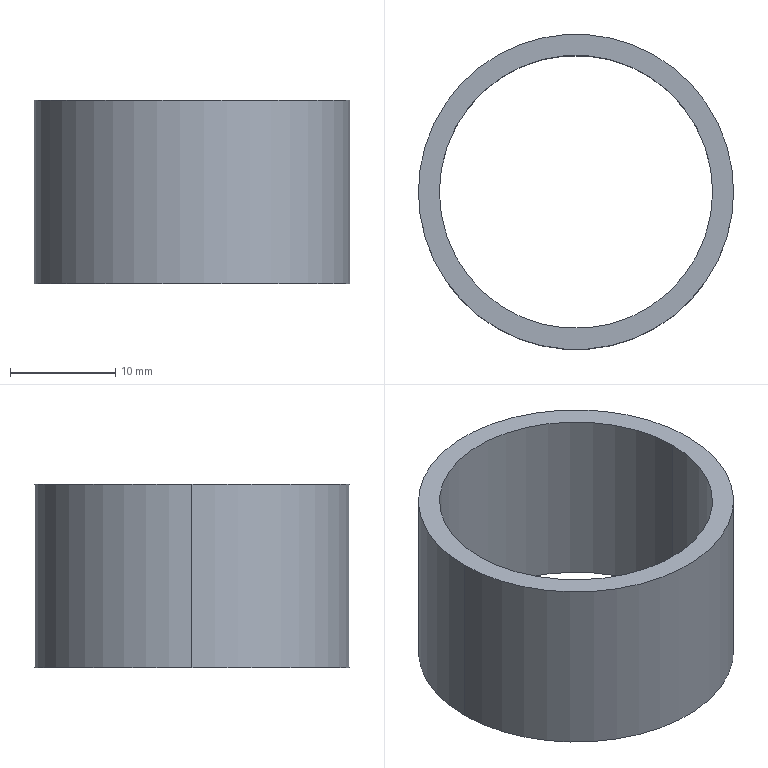Part | SolidWorks | features Extrusion 1 | 1 solid | 6 faces | box 30 x 30 x 17.5 mm | volume 3079 mm3 | cylinder 4 | plane 2 | commonest cylinder face diameters 26 x2 30 x2
STEP:
#1=CARTESIAN_POINT('',(-13.,0.,17.5));
#2=VERTEX_POINT('',#1);
#3=CARTESIAN_POINT('',(13.,0.,17.5));
#4=VERTEX_POINT('',#3);
#5=CARTESIAN_POINT('',(0.,0.,17.5));
#6=DIRECTION('',(0.,0.,1.));
#7=DIRECTION('',(1.,0.,0.));
#8=AXIS2_PLACEMENT_3D('',#5,#6,#7);
#9=CIRCLE('',#8,13.);
#10=EDGE_CURVE('',#2,#4,#9,.T.);
#11=ORIENTED_EDGE('',*,*,#10,.T.);
#12=CARTESIAN_POINT('',(13.,0.,0.));
#13=VERTEX_POINT('',#12);
#14=CARTESIAN_POINT('',(13.,0.,17.5));
#15=DIRECTION('',(0.,0.,-1.));
#16=VECTOR('',#15,1000.);
#17=LINE('',#14,#16);
#18=EDGE_CURVE('',#4,#13,#17,.T.);
#19=ORIENTED_EDGE('',*,*,#18,.T.);
#20=CARTESIAN_POINT('',(-13.,0.,0.));
#21=VERTEX_POINT('',#20);
#22=CARTESIAN_POINT('',(0.,0.,0.));
#23=DIRECTION('',(0.,0.,1.));
#24=DIRECTION('',(1.,0.,0.));
#25=AXIS2_PLACEMENT_3D('',#22,#23,#24);
#26=CIRCLE('',#25,13.);
#27=EDGE_CURVE('',#21,#13,#26,.T.);
#28=ORIENTED_EDGE('',*,*,#27,.F.);
#29=CARTESIAN_POINT('',(-13.,0.,17.5));
#30=DIRECTION('',(0.,0.,-1.));
#31=VECTOR('',#30,1000.);
#32=LINE('',#29,#31);
#33=EDGE_CURVE('',#2,#21,#32,.T.);
#34=ORIENTED_EDGE('',*,*,#33,.F.);
#35=EDGE_LOOP('',(#11,#19,#28,#34));
#36=FACE_OUTER_BOUND('',#35,.T.);
#37=CARTESIAN_POINT('',(0.,0.,17.5));
#38=DIRECTION('',(0.,0.,-1.));
#39=DIRECTION('',(-1.,0.,0.));
#40=AXIS2_PLACEMENT_3D('',#37,#38,#39);
#41=CYLINDRICAL_SURFACE('',#40,13.);
#42=ADVANCED_FACE('',(#36),#41,.F.);
#43=CARTESIAN_POINT('',(15.,0.,17.5));
#44=VERTEX_POINT('',#43);
#45=CARTESIAN_POINT('',(-15.,0.,17.5));
#46=VERTEX_POINT('',#45);
#47=CARTESIAN_POINT('',(0.,0.,17.5));
#48=DIRECTION('',(0.,0.,1.));
#49=DIRECTION('',(1.,0.,0.));
#50=AXIS2_PLACEMENT_3D('',#47,#48,#49);
#51=CIRCLE('',#50,15.);
#52=EDGE_CURVE('',#44,#46,#51,.T.);
#53=ORIENTED_EDGE('',*,*,#52,.F.);
#54=CARTESIAN_POINT('',(15.,0.,0.));
#55=VERTEX_POINT('',#54);
#56=CARTESIAN_POINT('',(15.,0.,17.5));
#57=DIRECTION('',(0.,0.,-1.));
#58=VECTOR('',#57,1000.);
#59=LINE('',#56,#58);
#60=EDGE_CURVE('',#44,#55,#59,.T.);
#61=ORIENTED_EDGE('',*,*,#60,.T.);
#62=CARTESIAN_POINT('',(-15.,0.,0.));
#63=VERTEX_POINT('',#62);
#64=CARTESIAN_POINT('',(0.,0.,0.));
#65=DIRECTION('',(0.,0.,1.));
#66=DIRECTION('',(1.,0.,0.));
#67=AXIS2_PLACEMENT_3D('',#64,#65,#66);
#68=CIRCLE('',#67,15.);
#69=EDGE_CURVE('',#55,#63,#68,.T.);
#70=ORIENTED_EDGE('',*,*,#69,.T.);
#71=CARTESIAN_POINT('',(-15.,0.,17.5));
#72=DIRECTION('',(0.,0.,-1.));
#73=VECTOR('',#72,1000.);
#74=LINE('',#71,#73);
#75=EDGE_CURVE('',#46,#63,#74,.T.);
#76=ORIENTED_EDGE('',*,*,#75,.F.);
#77=EDGE_LOOP('',(#53,#61,#70,#76));
#78=FACE_OUTER_BOUND('',#77,.T.);
#79=CARTESIAN_POINT('',(0.,0.,17.5));
#80=DIRECTION('',(0.,0.,-1.));
#81=DIRECTION('',(-1.,0.,0.));
#82=AXIS2_PLACEMENT_3D('',#79,#80,#81);
#83=CYLINDRICAL_SURFACE('',#82,15.);
#84=ADVANCED_FACE('',(#78),#83,.T.);
#85=CARTESIAN_POINT('',(0.,0.,17.5));
#86=DIRECTION('',(0.,0.,1.));
#87=DIRECTION('',(1.,0.,0.));
#88=AXIS2_PLACEMENT_3D('',#85,#86,#87);
#89=CIRCLE('',#88,15.);
#90=EDGE_CURVE('',#46,#44,#89,.T.);
#91=ORIENTED_EDGE('',*,*,#90,.T.);
#92=ORIENTED_EDGE('',*,*,#52,.T.);
#93=EDGE_LOOP('',(#91,#92));
#94=FACE_OUTER_BOUND('',#93,.T.);
#95=ORIENTED_EDGE('',*,*,#10,.F.);
#96=CARTESIAN_POINT('',(0.,0.,17.5));
#97=DIRECTION('',(0.,0.,1.));
#98=DIRECTION('',(1.,0.,0.));
#99=AXIS2_PLACEMENT_3D('',#96,#97,#98);
#100=CIRCLE('',#99,13.);
#101=EDGE_CURVE('',#4,#2,#100,.T.);
#102=ORIENTED_EDGE('',*,*,#101,.F.);
#103=EDGE_LOOP('',(#95,#102));
#104=FACE_BOUND('',#103,.T.);
#105=CARTESIAN_POINT('',(0.,0.,17.5));
#106=DIRECTION('',(0.,0.,1.));
#107=DIRECTION('',(1.,0.,0.));
#108=AXIS2_PLACEMENT_3D('',#105,#106,#107);
#109=PLANE('',#108);
#110=ADVANCED_FACE('',(#94,#104),#109,.T.);
#111=CARTESIAN_POINT('',(0.,0.,0.));
#112=DIRECTION('',(0.,0.,1.));
#113=DIRECTION('',(1.,0.,0.));
#114=AXIS2_PLACEMENT_3D('',#111,#112,#113);
#115=CIRCLE('',#114,15.);
#116=EDGE_CURVE('',#63,#55,#115,.T.);
#117=ORIENTED_EDGE('',*,*,#116,.F.);
#118=ORIENTED_EDGE('',*,*,#69,.F.);
#119=EDGE_LOOP('',(#117,#118));
#120=FACE_OUTER_BOUND('',#119,.T.);
#121=ORIENTED_EDGE('',*,*,#27,.T.);
#122=CARTESIAN_POINT('',(0.,0.,0.));
#123=DIRECTION('',(0.,0.,1.));
#124=DIRECTION('',(1.,0.,0.));
#125=AXIS2_PLACEMENT_3D('',#122,#123,#124);
#126=CIRCLE('',#125,13.);
#127=EDGE_CURVE('',#13,#21,#126,.T.);
#128=ORIENTED_EDGE('',*,*,#127,.T.);
#129=EDGE_LOOP('',(#121,#128));
#130=FACE_BOUND('',#129,.T.);
#131=CARTESIAN_POINT('',(0.,0.,0.));
#132=DIRECTION('',(0.,0.,1.));
#133=DIRECTION('',(1.,0.,0.));
#134=AXIS2_PLACEMENT_3D('',#131,#132,#133);
#135=PLANE('',#134);
#136=ADVANCED_FACE('',(#120,#130),#135,.F.);
#137=ORIENTED_EDGE('',*,*,#60,.F.);
#138=ORIENTED_EDGE('',*,*,#90,.F.);
#139=ORIENTED_EDGE('',*,*,#75,.T.);
#140=ORIENTED_EDGE('',*,*,#116,.T.);
#141=EDGE_LOOP('',(#137,#138,#139,#140));
#142=FACE_OUTER_BOUND('',#141,.T.);
#143=CARTESIAN_POINT('',(0.,0.,17.5));
#144=DIRECTION('',(0.,0.,-1.));
#145=DIRECTION('',(-1.,0.,0.));
#146=AXIS2_PLACEMENT_3D('',#143,#144,#145);
#147=CYLINDRICAL_SURFACE('',#146,15.);
#148=ADVANCED_FACE('',(#142),#147,.T.);
#149=ORIENTED_EDGE('',*,*,#18,.F.);
#150=ORIENTED_EDGE('',*,*,#101,.T.);
#151=ORIENTED_EDGE('',*,*,#33,.T.);
#152=ORIENTED_EDGE('',*,*,#127,.F.);
#153=EDGE_LOOP('',(#149,#150,#151,#152));
#154=FACE_OUTER_BOUND('',#153,.T.);
#155=CARTESIAN_POINT('',(0.,0.,17.5));
#156=DIRECTION('',(0.,0.,-1.));
#157=DIRECTION('',(-1.,0.,0.));
#158=AXIS2_PLACEMENT_3D('',#155,#156,#157);
#159=CYLINDRICAL_SURFACE('',#158,13.);
#160=ADVANCED_FACE('',(#154),#159,.F.);
#161=CLOSED_SHELL('',(#42,#84,#110,#136,#148,#160));
#162=MANIFOLD_SOLID_BREP('',#161);
#163=CARTESIAN_POINT('',(0.,0.,0.));
#164=DIRECTION('',(0.,0.,1.));
#165=DIRECTION('',(1.,0.,0.));
#166=AXIS2_PLACEMENT_3D('',#163,#164,#165);
#167=(LENGTH_UNIT()NAMED_UNIT(*)SI_UNIT(.MILLI.,.METRE.));
#168=UNCERTAINTY_MEASURE_WITH_UNIT(LENGTH_MEASURE(0.00001),#167,'','');
#169=(NAMED_UNIT(*)PLANE_ANGLE_UNIT()SI_UNIT($,.RADIAN.));
#170=(NAMED_UNIT(*)SI_UNIT($,.STERADIAN.)SOLID_ANGLE_UNIT());
#171=(GEOMETRIC_REPRESENTATION_CONTEXT(3)GLOBAL_UNCERTAINTY_ASSIGNED_CONTEXT((#168))GLOBAL_UNIT_ASSIGNED_CONTEXT((#167,#169,#170))REPRESENTATION_CONTEXT('',''));
#172=ADVANCED_BREP_SHAPE_REPRESENTATION('',(#162,#166),#171);